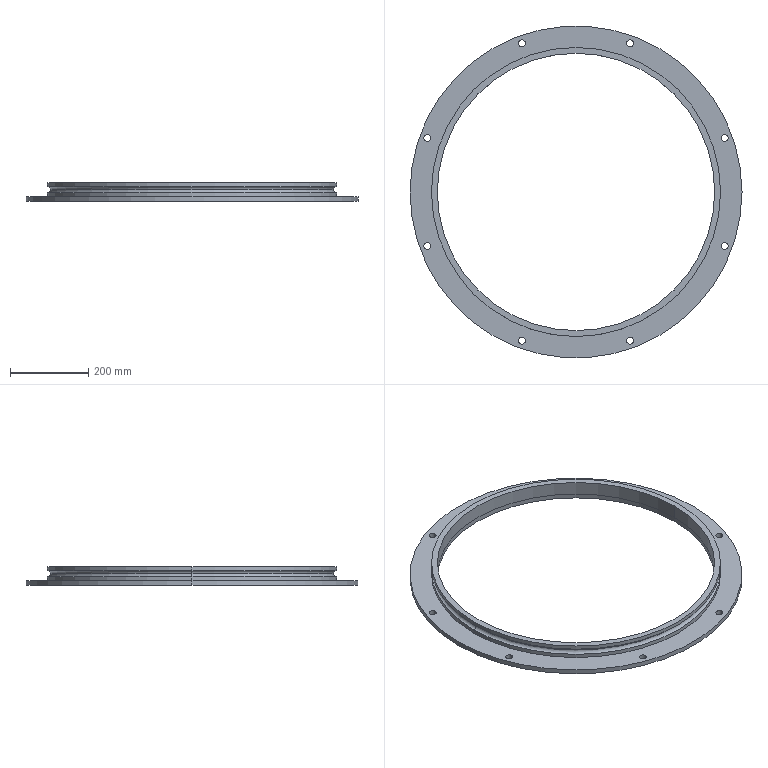Part | SolidWorks | features ICE 2, Extrusion 1, SweepCut 1 | 2 solids | 34 faces | box 850 x 850 x 48 mm | volume 3032308 mm3 | cylinder 26 | torus 4 | plane 4 | commonest cylinder face diameters 18 x16 710 x4 740 x4 850 x2
STEP:
#1=CARTESIAN_POINT('',(-370.,0.,22.));
#2=VERTEX_POINT('',#1);
#3=CARTESIAN_POINT('',(-362.,0.,30.));
#4=VERTEX_POINT('',#3);
#5=CARTESIAN_POINT('',(-370.,0.,30.));
#6=DIRECTION('',(0.,-1.,0.));
#7=DIRECTION('',(0.,0.,-1.));
#8=AXIS2_PLACEMENT_3D('',#5,#6,#7);
#9=CIRCLE('',#8,8.);
#10=EDGE_CURVE('',#2,#4,#9,.T.);
#11=ORIENTED_EDGE('',*,*,#10,.T.);
#12=CARTESIAN_POINT('',(362.,0.,30.));
#13=VERTEX_POINT('',#12);
#14=CARTESIAN_POINT('',(0.,0.,30.));
#15=DIRECTION('',(0.,0.,-1.));
#16=DIRECTION('',(-1.,0.,0.));
#17=AXIS2_PLACEMENT_3D('',#14,#15,#16);
#18=CIRCLE('',#17,362.);
#19=EDGE_CURVE('',#4,#13,#18,.T.);
#20=ORIENTED_EDGE('',*,*,#19,.T.);
#21=CARTESIAN_POINT('',(370.,0.,22.));
#22=VERTEX_POINT('',#21);
#23=CARTESIAN_POINT('',(370.,0.,30.));
#24=DIRECTION('',(0.,1.,0.));
#25=DIRECTION('',(-1.,0.,0.));
#26=AXIS2_PLACEMENT_3D('',#23,#24,#25);
#27=CIRCLE('',#26,8.);
#28=EDGE_CURVE('',#22,#13,#27,.T.);
#29=ORIENTED_EDGE('',*,*,#28,.F.);
#30=CARTESIAN_POINT('',(0.,0.,22.));
#31=DIRECTION('',(0.,0.,-1.));
#32=DIRECTION('',(1.,0.,0.));
#33=AXIS2_PLACEMENT_3D('',#30,#31,#32);
#34=CIRCLE('',#33,370.);
#35=EDGE_CURVE('',#2,#22,#34,.T.);
#36=ORIENTED_EDGE('',*,*,#35,.F.);
#37=EDGE_LOOP('',(#11,#20,#29,#36));
#38=FACE_OUTER_BOUND('',#37,.T.);
#39=CARTESIAN_POINT('',(0.,0.,30.));
#40=DIRECTION('',(0.,0.,-1.));
#41=DIRECTION('',(-1.,0.,0.));
#42=AXIS2_PLACEMENT_3D('',#39,#40,#41);
#43=TOROIDAL_SURFACE('',#42,370.,8.);
#44=ADVANCED_FACE('',(#38),#43,.F.);
#45=ORIENTED_EDGE('',*,*,#28,.T.);
#46=CARTESIAN_POINT('',(0.,0.,30.));
#47=DIRECTION('',(0.,0.,-1.));
#48=DIRECTION('',(-1.,0.,0.));
#49=AXIS2_PLACEMENT_3D('',#46,#47,#48);
#50=CIRCLE('',#49,362.);
#51=EDGE_CURVE('',#13,#4,#50,.T.);
#52=ORIENTED_EDGE('',*,*,#51,.T.);
#53=ORIENTED_EDGE('',*,*,#10,.F.);
#54=CARTESIAN_POINT('',(0.,0.,22.));
#55=DIRECTION('',(0.,0.,-1.));
#56=DIRECTION('',(1.,0.,0.));
#57=AXIS2_PLACEMENT_3D('',#54,#55,#56);
#58=CIRCLE('',#57,370.);
#59=EDGE_CURVE('',#22,#2,#58,.T.);
#60=ORIENTED_EDGE('',*,*,#59,.F.);
#61=EDGE_LOOP('',(#45,#52,#53,#60));
#62=FACE_OUTER_BOUND('',#61,.T.);
#63=CARTESIAN_POINT('',(0.,0.,30.));
#64=DIRECTION('',(0.,0.,-1.));
#65=DIRECTION('',(-1.,0.,0.));
#66=AXIS2_PLACEMENT_3D('',#63,#64,#65);
#67=TOROIDAL_SURFACE('',#66,370.,8.);
#68=ADVANCED_FACE('',(#62),#67,.F.);
#69=ORIENTED_EDGE('',*,*,#51,.F.);
#70=CARTESIAN_POINT('',(370.,0.,38.));
#71=VERTEX_POINT('',#70);
#72=CARTESIAN_POINT('',(370.,0.,30.));
#73=DIRECTION('',(0.,1.,0.));
#74=DIRECTION('',(-1.,0.,0.));
#75=AXIS2_PLACEMENT_3D('',#72,#73,#74);
#76=CIRCLE('',#75,8.);
#77=EDGE_CURVE('',#13,#71,#76,.T.);
#78=ORIENTED_EDGE('',*,*,#77,.T.);
#79=CARTESIAN_POINT('',(-370.,0.,38.));
#80=VERTEX_POINT('',#79);
#81=CARTESIAN_POINT('',(0.,0.,38.));
#82=DIRECTION('',(0.,0.,1.));
#83=DIRECTION('',(-1.,0.,0.));
#84=AXIS2_PLACEMENT_3D('',#81,#82,#83);
#85=CIRCLE('',#84,370.);
#86=EDGE_CURVE('',#80,#71,#85,.T.);
#87=ORIENTED_EDGE('',*,*,#86,.F.);
#88=CARTESIAN_POINT('',(-370.,0.,30.));
#89=DIRECTION('',(0.,-1.,0.));
#90=DIRECTION('',(0.,0.,-1.));
#91=AXIS2_PLACEMENT_3D('',#88,#89,#90);
#92=CIRCLE('',#91,8.);
#93=EDGE_CURVE('',#4,#80,#92,.T.);
#94=ORIENTED_EDGE('',*,*,#93,.F.);
#95=EDGE_LOOP('',(#69,#78,#87,#94));
#96=FACE_OUTER_BOUND('',#95,.T.);
#97=CARTESIAN_POINT('',(0.,0.,30.));
#98=DIRECTION('',(0.,0.,-1.));
#99=DIRECTION('',(-1.,0.,0.));
#100=AXIS2_PLACEMENT_3D('',#97,#98,#99);
#101=TOROIDAL_SURFACE('',#100,370.,8.);
#102=ADVANCED_FACE('',(#96),#101,.F.);
#103=CARTESIAN_POINT('',(-355.,0.,48.));
#104=VERTEX_POINT('',#103);
#105=CARTESIAN_POINT('',(355.,0.,48.));
#106=VERTEX_POINT('',#105);
#107=CARTESIAN_POINT('',(0.,0.,48.));
#108=DIRECTION('',(0.,0.,1.));
#109=DIRECTION('',(1.,0.,0.));
#110=AXIS2_PLACEMENT_3D('',#107,#108,#109);
#111=CIRCLE('',#110,355.);
#112=EDGE_CURVE('',#104,#106,#111,.T.);
#113=ORIENTED_EDGE('',*,*,#112,.T.);
#114=CARTESIAN_POINT('',(355.,0.,12.));
#115=VERTEX_POINT('',#114);
#116=CARTESIAN_POINT('',(355.,0.,48.));
#117=DIRECTION('',(0.,0.,-1.));
#118=VECTOR('',#117,1000.);
#119=LINE('',#116,#118);
#120=EDGE_CURVE('',#106,#115,#119,.T.);
#121=ORIENTED_EDGE('',*,*,#120,.T.);
#122=CARTESIAN_POINT('',(-355.,0.,12.));
#123=VERTEX_POINT('',#122);
#124=CARTESIAN_POINT('',(0.,0.,12.));
#125=DIRECTION('',(0.,0.,1.));
#126=DIRECTION('',(1.,0.,0.));
#127=AXIS2_PLACEMENT_3D('',#124,#125,#126);
#128=CIRCLE('',#127,355.);
#129=EDGE_CURVE('',#123,#115,#128,.T.);
#130=ORIENTED_EDGE('',*,*,#129,.F.);
#131=CARTESIAN_POINT('',(-355.,0.,48.));
#132=DIRECTION('',(0.,0.,-1.));
#133=VECTOR('',#132,1000.);
#134=LINE('',#131,#133);
#135=EDGE_CURVE('',#104,#123,#134,.T.);
#136=ORIENTED_EDGE('',*,*,#135,.F.);
#137=EDGE_LOOP('',(#113,#121,#130,#136));
#138=FACE_OUTER_BOUND('',#137,.T.);
#139=CARTESIAN_POINT('',(0.,0.,48.));
#140=DIRECTION('',(0.,0.,-1.));
#141=DIRECTION('',(-1.,0.,0.));
#142=AXIS2_PLACEMENT_3D('',#139,#140,#141);
#143=CYLINDRICAL_SURFACE('',#142,355.);
#144=ADVANCED_FACE('',(#138),#143,.F.);
#145=CARTESIAN_POINT('',(370.,0.,48.));
#146=VERTEX_POINT('',#145);
#147=CARTESIAN_POINT('',(-370.,0.,48.));
#148=VERTEX_POINT('',#147);
#149=CARTESIAN_POINT('',(0.,0.,48.));
#150=DIRECTION('',(0.,0.,1.));
#151=DIRECTION('',(1.,0.,0.));
#152=AXIS2_PLACEMENT_3D('',#149,#150,#151);
#153=CIRCLE('',#152,370.);
#154=EDGE_CURVE('',#146,#148,#153,.T.);
#155=ORIENTED_EDGE('',*,*,#154,.F.);
#156=CARTESIAN_POINT('',(370.,0.,48.));
#157=DIRECTION('',(0.,0.,-1.));
#158=VECTOR('',#157,1000.);
#159=LINE('',#156,#158);
#160=EDGE_CURVE('',#146,#71,#159,.T.);
#161=ORIENTED_EDGE('',*,*,#160,.T.);
#162=CARTESIAN_POINT('',(0.,0.,38.));
#163=DIRECTION('',(0.,0.,1.));
#164=DIRECTION('',(-1.,0.,0.));
#165=AXIS2_PLACEMENT_3D('',#162,#163,#164);
#166=CIRCLE('',#165,370.);
#167=EDGE_CURVE('',#71,#80,#166,.T.);
#168=ORIENTED_EDGE('',*,*,#167,.T.);
#169=CARTESIAN_POINT('',(-370.,0.,48.));
#170=DIRECTION('',(0.,0.,-1.));
#171=VECTOR('',#170,1000.);
#172=LINE('',#169,#171);
#173=EDGE_CURVE('',#148,#80,#172,.T.);
#174=ORIENTED_EDGE('',*,*,#173,.F.);
#175=EDGE_LOOP('',(#155,#161,#168,#174));
#176=FACE_OUTER_BOUND('',#175,.T.);
#177=CARTESIAN_POINT('',(0.,0.,48.));
#178=DIRECTION('',(0.,0.,-1.));
#179=DIRECTION('',(-1.,0.,0.));
#180=AXIS2_PLACEMENT_3D('',#177,#178,#179);
#181=CYLINDRICAL_SURFACE('',#180,370.);
#182=ADVANCED_FACE('',(#176),#181,.T.);
#183=ORIENTED_EDGE('',*,*,#35,.T.);
#184=CARTESIAN_POINT('',(370.,0.,12.));
#185=VERTEX_POINT('',#184);
#186=CARTESIAN_POINT('',(370.,0.,48.));
#187=DIRECTION('',(0.,0.,-1.));
#188=VECTOR('',#187,1000.);
#189=LINE('',#186,#188);
#190=EDGE_CURVE('',#22,#185,#189,.T.);
#191=ORIENTED_EDGE('',*,*,#190,.T.);
#192=CARTESIAN_POINT('',(-370.,0.,12.));
#193=VERTEX_POINT('',#192);
#194=CARTESIAN_POINT('',(0.,0.,12.));
#195=DIRECTION('',(0.,0.,1.));
#196=DIRECTION('',(1.,0.,0.));
#197=AXIS2_PLACEMENT_3D('',#194,#195,#196);
#198=CIRCLE('',#197,370.);
#199=EDGE_CURVE('',#185,#193,#198,.T.);
#200=ORIENTED_EDGE('',*,*,#199,.T.);
#201=CARTESIAN_POINT('',(-370.,0.,48.));
#202=DIRECTION('',(0.,0.,-1.));
#203=VECTOR('',#202,1000.);
#204=LINE('',#201,#203);
#205=EDGE_CURVE('',#2,#193,#204,.T.);
#206=ORIENTED_EDGE('',*,*,#205,.F.);
#207=EDGE_LOOP('',(#183,#191,#200,#206));
#208=FACE_OUTER_BOUND('',#207,.T.);
#209=CARTESIAN_POINT('',(0.,0.,48.));
#210=DIRECTION('',(0.,0.,-1.));
#211=DIRECTION('',(-1.,0.,0.));
#212=AXIS2_PLACEMENT_3D('',#209,#210,#211);
#213=CYLINDRICAL_SURFACE('',#212,370.);
#214=ADVANCED_FACE('',(#208),#213,.T.);
#215=ORIENTED_EDGE('',*,*,#190,.F.);
#216=ORIENTED_EDGE('',*,*,#59,.T.);
#217=ORIENTED_EDGE('',*,*,#205,.T.);
#218=CARTESIAN_POINT('',(0.,0.,12.));
#219=DIRECTION('',(0.,0.,1.));
#220=DIRECTION('',(1.,0.,0.));
#221=AXIS2_PLACEMENT_3D('',#218,#219,#220);
#222=CIRCLE('',#221,370.);
#223=EDGE_CURVE('',#193,#185,#222,.T.);
#224=ORIENTED_EDGE('',*,*,#223,.T.);
#225=EDGE_LOOP('',(#215,#216,#217,#224));
#226=FACE_OUTER_BOUND('',#225,.T.);
#227=CARTESIAN_POINT('',(0.,0.,48.));
#228=DIRECTION('',(0.,0.,-1.));
#229=DIRECTION('',(-1.,0.,0.));
#230=AXIS2_PLACEMENT_3D('',#227,#228,#229);
#231=CYLINDRICAL_SURFACE('',#230,370.);
#232=ADVANCED_FACE('',(#226),#231,.T.);
#233=CARTESIAN_POINT('',(0.,0.,48.));
#234=DIRECTION('',(0.,0.,1.));
#235=DIRECTION('',(1.,0.,0.));
#236=AXIS2_PLACEMENT_3D('',#233,#234,#235);
#237=CIRCLE('',#236,370.);
#238=EDGE_CURVE('',#148,#146,#237,.T.);
#239=ORIENTED_EDGE('',*,*,#238,.T.);
#240=ORIENTED_EDGE('',*,*,#154,.T.);
#241=EDGE_LOOP('',(#239,#240));
#242=FACE_OUTER_BOUND('',#241,.T.);
#243=ORIENTED_EDGE('',*,*,#112,.F.);
#244=CARTESIAN_POINT('',(0.,0.,48.));
#245=DIRECTION('',(0.,0.,1.));
#246=DIRECTION('',(1.,0.,0.));
#247=AXIS2_PLACEMENT_3D('',#244,#245,#246);
#248=CIRCLE('',#247,355.);
#249=EDGE_CURVE('',#106,#104,#248,.T.);
#250=ORIENTED_EDGE('',*,*,#249,.F.);
#251=EDGE_LOOP('',(#243,#250));
#252=FACE_BOUND('',#251,.T.);
#253=CARTESIAN_POINT('',(0.,0.,48.));
#254=DIRECTION('',(0.,0.,1.));
#255=DIRECTION('',(1.,0.,0.));
#256=AXIS2_PLACEMENT_3D('',#253,#254,#255);
#257=PLANE('',#256);
#258=ADVANCED_FACE('',(#242,#252),#257,.T.);
#259=ORIENTED_EDGE('',*,*,#223,.F.);
#260=ORIENTED_EDGE('',*,*,#199,.F.);
#261=EDGE_LOOP('',(#259,#260));
#262=FACE_OUTER_BOUND('',#261,.T.);
#263=ORIENTED_EDGE('',*,*,#129,.T.);
#264=CARTESIAN_POINT('',(0.,0.,12.));
#265=DIRECTION('',(0.,0.,1.));
#266=DIRECTION('',(1.,0.,0.));
#267=AXIS2_PLACEMENT_3D('',#264,#265,#266);
#268=CIRCLE('',#267,355.);
#269=EDGE_CURVE('',#115,#123,#268,.T.);
#270=ORIENTED_EDGE('',*,*,#269,.T.);
#271=EDGE_LOOP('',(#263,#270));
#272=FACE_BOUND('',#271,.T.);
#273=CARTESIAN_POINT('',(0.,0.,12.));
#274=DIRECTION('',(0.,0.,1.));
#275=DIRECTION('',(1.,0.,0.));
#276=AXIS2_PLACEMENT_3D('',#273,#274,#275);
#277=PLANE('',#276);
#278=ADVANCED_FACE('',(#262,#272),#277,.F.);
#279=ORIENTED_EDGE('',*,*,#160,.F.);
#280=ORIENTED_EDGE('',*,*,#238,.F.);
#281=ORIENTED_EDGE('',*,*,#173,.T.);
#282=ORIENTED_EDGE('',*,*,#86,.T.);
#283=EDGE_LOOP('',(#279,#280,#281,#282));
#284=FACE_OUTER_BOUND('',#283,.T.);
#285=CARTESIAN_POINT('',(0.,0.,48.));
#286=DIRECTION('',(0.,0.,-1.));
#287=DIRECTION('',(-1.,0.,0.));
#288=AXIS2_PLACEMENT_3D('',#285,#286,#287);
#289=CYLINDRICAL_SURFACE('',#288,370.);
#290=ADVANCED_FACE('',(#284),#289,.T.);
#291=ORIENTED_EDGE('',*,*,#120,.F.);
#292=ORIENTED_EDGE('',*,*,#249,.T.);
#293=ORIENTED_EDGE('',*,*,#135,.T.);
#294=ORIENTED_EDGE('',*,*,#269,.F.);
#295=EDGE_LOOP('',(#291,#292,#293,#294));
#296=FACE_OUTER_BOUND('',#295,.T.);
#297=CARTESIAN_POINT('',(0.,0.,48.));
#298=DIRECTION('',(0.,0.,-1.));
#299=DIRECTION('',(-1.,0.,0.));
#300=AXIS2_PLACEMENT_3D('',#297,#298,#299);
#301=CYLINDRICAL_SURFACE('',#300,355.);
#302=ADVANCED_FACE('',(#296),#301,.F.);
#303=ORIENTED_EDGE('',*,*,#19,.F.);
#304=ORIENTED_EDGE('',*,*,#93,.T.);
#305=ORIENTED_EDGE('',*,*,#167,.F.);
#306=ORIENTED_EDGE('',*,*,#77,.F.);
#307=EDGE_LOOP('',(#303,#304,#305,#306));
#308=FACE_OUTER_BOUND('',#307,.T.);
#309=CARTESIAN_POINT('',(0.,0.,30.));
#310=DIRECTION('',(0.,0.,-1.));
#311=DIRECTION('',(-1.,0.,0.));
#312=AXIS2_PLACEMENT_3D('',#309,#310,#311);
#313=TOROIDAL_SURFACE('',#312,370.,8.);
#314=ADVANCED_FACE('',(#308),#313,.F.);
#315=CLOSED_SHELL('',(#44,#68,#102,#144,#182,#214,#232,#258,#278,#290,#302,#314));
#316=MANIFOLD_SOLID_BREP('',#315);
#317=CARTESIAN_POINT('',(129.5,380.582,0.));
#318=VERTEX_POINT('',#317);
#319=CARTESIAN_POINT('',(147.5,380.582,0.));
#320=VERTEX_POINT('',#319);
#321=CARTESIAN_POINT('',(138.5,380.582,0.));
#322=DIRECTION('',(0.,0.,1.));
#323=DIRECTION('',(1.,0.,0.));
#324=AXIS2_PLACEMENT_3D('',#321,#322,#323);
#325=CIRCLE('',#324,9.);
#326=EDGE_CURVE('',#318,#320,#325,.T.);
#327=ORIENTED_EDGE('',*,*,#326,.F.);
#328=CARTESIAN_POINT('',(129.5,380.582,12.));
#329=VERTEX_POINT('',#328);
#330=CARTESIAN_POINT('',(129.5,380.582,-8.));
#331=DIRECTION('',(0.,0.,1.));
#332=VECTOR('',#331,1000.);
#333=LINE('',#330,#332);
#334=EDGE_CURVE('',#318,#329,#333,.T.);
#335=ORIENTED_EDGE('',*,*,#334,.T.);
#336=CARTESIAN_POINT('',(147.5,380.582,12.));
#337=VERTEX_POINT('',#336);
#338=CARTESIAN_POINT('',(138.5,380.582,12.));
#339=DIRECTION('',(0.,0.,1.));
#340=DIRECTION('',(1.,0.,0.));
#341=AXIS2_PLACEMENT_3D('',#338,#339,#340);
#342=CIRCLE('',#341,9.);
#343=EDGE_CURVE('',#329,#337,#342,.T.);
#344=ORIENTED_EDGE('',*,*,#343,.T.);
#345=CARTESIAN_POINT('',(147.5,380.582,-8.));
#346=DIRECTION('',(0.,0.,1.));
#347=VECTOR('',#346,1000.);
#348=LINE('',#345,#347);
#349=EDGE_CURVE('',#320,#337,#348,.T.);
#350=ORIENTED_EDGE('',*,*,#349,.F.);
#351=EDGE_LOOP('',(#327,#335,#344,#350));
#352=FACE_OUTER_BOUND('',#351,.T.);
#353=CARTESIAN_POINT('',(138.5,380.582,-8.));
#354=DIRECTION('',(0.,0.,1.));
#355=DIRECTION('',(1.,0.,0.));
#356=AXIS2_PLACEMENT_3D('',#353,#354,#355);
#357=CYLINDRICAL_SURFACE('',#356,9.);
#358=ADVANCED_FACE('',(#352),#357,.F.);
#359=CARTESIAN_POINT('',(129.5,-380.582,0.));
#360=VERTEX_POINT('',#359);
#361=CARTESIAN_POINT('',(147.5,-380.582,0.));
#362=VERTEX_POINT('',#361);
#363=CARTESIAN_POINT('',(138.5,-380.582,0.));
#364=DIRECTION('',(0.,0.,1.));
#365=DIRECTION('',(1.,0.,0.));
#366=AXIS2_PLACEMENT_3D('',#363,#364,#365);
#367=CIRCLE('',#366,9.);
#368=EDGE_CURVE('',#360,#362,#367,.T.);
#369=ORIENTED_EDGE('',*,*,#368,.F.);
#370=CARTESIAN_POINT('',(129.5,-380.582,12.));
#371=VERTEX_POINT('',#370);
#372=CARTESIAN_POINT('',(129.5,-380.582,-8.));
#373=DIRECTION('',(0.,0.,1.));
#374=VECTOR('',#373,1000.);
#375=LINE('',#372,#374);
#376=EDGE_CURVE('',#360,#371,#375,.T.);
#377=ORIENTED_EDGE('',*,*,#376,.T.);
#378=CARTESIAN_POINT('',(147.5,-380.582,12.));
#379=VERTEX_POINT('',#378);
#380=CARTESIAN_POINT('',(138.5,-380.582,12.));
#381=DIRECTION('',(0.,0.,1.));
#382=DIRECTION('',(-1.,0.,0.));
#383=AXIS2_PLACEMENT_3D('',#380,#381,#382);
#384=CIRCLE('',#383,9.);
#385=EDGE_CURVE('',#371,#379,#384,.T.);
#386=ORIENTED_EDGE('',*,*,#385,.T.);
#387=CARTESIAN_POINT('',(147.5,-380.582,-8.));
#388=DIRECTION('',(0.,0.,1.));
#389=VECTOR('',#388,1000.);
#390=LINE('',#387,#389);
#391=EDGE_CURVE('',#362,#379,#390,.T.);
#392=ORIENTED_EDGE('',*,*,#391,.F.);
#393=EDGE_LOOP('',(#369,#377,#386,#392));
#394=FACE_OUTER_BOUND('',#393,.T.);
#395=CARTESIAN_POINT('',(138.5,-380.582,-8.));
#396=DIRECTION('',(0.,0.,1.));
#397=DIRECTION('',(1.,0.,0.));
#398=AXIS2_PLACEMENT_3D('',#395,#396,#397);
#399=CYLINDRICAL_SURFACE('',#398,9.);
#400=ADVANCED_FACE('',(#394),#399,.F.);
#401=CARTESIAN_POINT('',(-147.5,-380.582,0.));
#402=VERTEX_POINT('',#401);
#403=CARTESIAN_POINT('',(-129.5,-380.582,0.));
#404=VERTEX_POINT('',#403);
#405=CARTESIAN_POINT('',(-138.5,-380.582,0.));
#406=DIRECTION('',(0.,0.,1.));
#407=DIRECTION('',(1.,0.,0.));
#408=AXIS2_PLACEMENT_3D('',#405,#406,#407);
#409=CIRCLE('',#408,9.);
#410=EDGE_CURVE('',#402,#404,#409,.T.);
#411=ORIENTED_EDGE('',*,*,#410,.F.);
#412=CARTESIAN_POINT('',(-147.5,-380.582,12.));
#413=VERTEX_POINT('',#412);
#414=CARTESIAN_POINT('',(-147.5,-380.582,-8.));
#415=DIRECTION('',(0.,0.,1.));
#416=VECTOR('',#415,1000.);
#417=LINE('',#414,#416);
#418=EDGE_CURVE('',#402,#413,#417,.T.);
#419=ORIENTED_EDGE('',*,*,#418,.T.);
#420=CARTESIAN_POINT('',(-129.5,-380.582,12.));
#421=VERTEX_POINT('',#420);
#422=CARTESIAN_POINT('',(-138.5,-380.582,12.));
#423=DIRECTION('',(0.,0.,1.));
#424=DIRECTION('',(-1.,0.,0.));
#425=AXIS2_PLACEMENT_3D('',#422,#423,#424);
#426=CIRCLE('',#425,9.);
#427=EDGE_CURVE('',#413,#421,#426,.T.);
#428=ORIENTED_EDGE('',*,*,#427,.T.);
#429=CARTESIAN_POINT('',(-129.5,-380.582,-8.));
#430=DIRECTION('',(0.,0.,1.));
#431=VECTOR('',#430,1000.);
#432=LINE('',#429,#431);
#433=EDGE_CURVE('',#404,#421,#432,.T.);
#434=ORIENTED_EDGE('',*,*,#433,.F.);
#435=EDGE_LOOP('',(#411,#419,#428,#434));
#436=FACE_OUTER_BOUND('',#435,.T.);
#437=CARTESIAN_POINT('',(-138.5,-380.582,-8.));
#438=DIRECTION('',(0.,0.,1.));
#439=DIRECTION('',(1.,0.,0.));
#440=AXIS2_PLACEMENT_3D('',#437,#438,#439);
#441=CYLINDRICAL_SURFACE('',#440,9.);
#442=ADVANCED_FACE('',(#436),#441,.F.);
#443=CARTESIAN_POINT('',(-389.582,138.5,0.));
#444=VERTEX_POINT('',#443);
#445=CARTESIAN_POINT('',(-371.582,138.5,0.));
#446=VERTEX_POINT('',#445);
#447=CARTESIAN_POINT('',(-380.582,138.5,0.));
#448=DIRECTION('',(0.,0.,1.));
#449=DIRECTION('',(1.,0.,0.));
#450=AXIS2_PLACEMENT_3D('',#447,#448,#449);
#451=CIRCLE('',#450,9.);
#452=EDGE_CURVE('',#444,#446,#451,.T.);
#453=ORIENTED_EDGE('',*,*,#452,.F.);
#454=CARTESIAN_POINT('',(-389.582,138.5,12.));
#455=VERTEX_POINT('',#454);
#456=CARTESIAN_POINT('',(-389.582,138.5,-8.));
#457=DIRECTION('',(0.,0.,1.));
#458=VECTOR('',#457,1000.);
#459=LINE('',#456,#458);
#460=EDGE_CURVE('',#444,#455,#459,.T.);
#461=ORIENTED_EDGE('',*,*,#460,.T.);
#462=CARTESIAN_POINT('',(-371.582,138.5,12.));
#463=VERTEX_POINT('',#462);
#464=CARTESIAN_POINT('',(-380.582,138.5,12.));
#465=DIRECTION('',(0.,0.,1.));
#466=DIRECTION('',(1.,0.,0.));
#467=AXIS2_PLACEMENT_3D('',#464,#465,#466);
#468=CIRCLE('',#467,9.);
#469=EDGE_CURVE('',#455,#463,#468,.T.);
#470=ORIENTED_EDGE('',*,*,#469,.T.);
#471=CARTESIAN_POINT('',(-371.582,138.5,-8.));
#472=DIRECTION('',(0.,0.,1.));
#473=VECTOR('',#472,1000.);
#474=LINE('',#471,#473);
#475=EDGE_CURVE('',#446,#463,#474,.T.);
#476=ORIENTED_EDGE('',*,*,#475,.F.);
#477=EDGE_LOOP('',(#453,#461,#470,#476));
#478=FACE_OUTER_BOUND('',#477,.T.);
#479=CARTESIAN_POINT('',(-380.582,138.5,-8.));
#480=DIRECTION('',(0.,0.,1.));
#481=DIRECTION('',(1.,0.,0.));
#482=AXIS2_PLACEMENT_3D('',#479,#480,#481);
#483=CYLINDRICAL_SURFACE('',#482,9.);
#484=ADVANCED_FACE('',(#478),#483,.F.);
#485=CARTESIAN_POINT('',(-389.582,-138.5,0.));
#486=VERTEX_POINT('',#485);
#487=CARTESIAN_POINT('',(-371.582,-138.5,0.));
#488=VERTEX_POINT('',#487);
#489=CARTESIAN_POINT('',(-380.582,-138.5,0.));
#490=DIRECTION('',(0.,0.,1.));
#491=DIRECTION('',(1.,0.,0.));
#492=AXIS2_PLACEMENT_3D('',#489,#490,#491);
#493=CIRCLE('',#492,9.);
#494=EDGE_CURVE('',#486,#488,#493,.T.);
#495=ORIENTED_EDGE('',*,*,#494,.F.);
#496=CARTESIAN_POINT('',(-389.582,-138.5,12.));
#497=VERTEX_POINT('',#496);
#498=CARTESIAN_POINT('',(-389.582,-138.5,-8.));
#499=DIRECTION('',(0.,0.,1.));
#500=VECTOR('',#499,1000.);
#501=LINE('',#498,#500);
#502=EDGE_CURVE('',#486,#497,#501,.T.);
#503=ORIENTED_EDGE('',*,*,#502,.T.);
#504=CARTESIAN_POINT('',(-371.582,-138.5,12.));
#505=VERTEX_POINT('',#504);
#506=CARTESIAN_POINT('',(-380.582,-138.5,12.));
#507=DIRECTION('',(0.,0.,1.));
#508=DIRECTION('',(1.,0.,0.));
#509=AXIS2_PLACEMENT_3D('',#506,#507,#508);
#510=CIRCLE('',#509,9.);
#511=EDGE_CURVE('',#497,#505,#510,.T.);
#512=ORIENTED_EDGE('',*,*,#511,.T.);
#513=CARTESIAN_POINT('',(-371.582,-138.5,-8.));
#514=DIRECTION('',(0.,0.,1.));
#515=VECTOR('',#514,1000.);
#516=LINE('',#513,#515);
#517=EDGE_CURVE('',#488,#505,#516,.T.);
#518=ORIENTED_EDGE('',*,*,#517,.F.);
#519=EDGE_LOOP('',(#495,#503,#512,#518));
#520=FACE_OUTER_BOUND('',#519,.T.);
#521=CARTESIAN_POINT('',(-380.582,-138.5,-8.));
#522=DIRECTION('',(0.,0.,1.));
#523=DIRECTION('',(1.,0.,0.));
#524=AXIS2_PLACEMENT_3D('',#521,#522,#523);
#525=CYLINDRICAL_SURFACE('',#524,9.);
#526=ADVANCED_FACE('',(#520),#525,.F.);
#527=CARTESIAN_POINT('',(371.582,-138.5,0.));
#528=VERTEX_POINT('',#527);
#529=CARTESIAN_POINT('',(389.582,-138.5,0.));
#530=VERTEX_POINT('',#529);
#531=CARTESIAN_POINT('',(380.582,-138.5,0.));
#532=DIRECTION('',(0.,0.,1.));
#533=DIRECTION('',(1.,0.,0.));
#534=AXIS2_PLACEMENT_3D('',#531,#532,#533);
#535=CIRCLE('',#534,9.);
#536=EDGE_CURVE('',#528,#530,#535,.T.);
#537=ORIENTED_EDGE('',*,*,#536,.F.);
#538=CARTESIAN_POINT('',(371.582,-138.5,12.));
#539=VERTEX_POINT('',#538);
#540=CARTESIAN_POINT('',(371.582,-138.5,-8.));
#541=DIRECTION('',(0.,0.,1.));
#542=VECTOR('',#541,1000.);
#543=LINE('',#540,#542);
#544=EDGE_CURVE('',#528,#539,#543,.T.);
#545=ORIENTED_EDGE('',*,*,#544,.T.);
#546=CARTESIAN_POINT('',(389.582,-138.5,12.));
#547=VERTEX_POINT('',#546);
#548=CARTESIAN_POINT('',(380.582,-138.5,12.));
#549=DIRECTION('',(0.,0.,1.));
#550=DIRECTION('',(-1.,0.,0.));
#551=AXIS2_PLACEMENT_3D('',#548,#549,#550);
#552=CIRCLE('',#551,9.);
#553=EDGE_CURVE('',#539,#547,#552,.T.);
#554=ORIENTED_EDGE('',*,*,#553,.T.);
#555=CARTESIAN_POINT('',(389.582,-138.5,-8.));
#556=DIRECTION('',(0.,0.,1.));
#557=VECTOR('',#556,1000.);
#558=LINE('',#555,#557);
#559=EDGE_CURVE('',#530,#547,#558,.T.);
#560=ORIENTED_EDGE('',*,*,#559,.F.);
#561=EDGE_LOOP('',(#537,#545,#554,#560));
#562=FACE_OUTER_BOUND('',#561,.T.);
#563=CARTESIAN_POINT('',(380.582,-138.5,-8.));
#564=DIRECTION('',(0.,0.,1.));
#565=DIRECTION('',(1.,0.,0.));
#566=AXIS2_PLACEMENT_3D('',#563,#564,#565);
#567=CYLINDRICAL_SURFACE('',#566,9.);
#568=ADVANCED_FACE('',(#562),#567,.F.);
#569=CARTESIAN_POINT('',(371.582,138.5,0.));
#570=VERTEX_POINT('',#569);
#571=CARTESIAN_POINT('',(389.582,138.5,0.));
#572=VERTEX_POINT('',#571);
#573=CARTESIAN_POINT('',(380.582,138.5,0.));
#574=DIRECTION('',(0.,0.,1.));
#575=DIRECTION('',(1.,0.,0.));
#576=AXIS2_PLACEMENT_3D('',#573,#574,#575);
#577=CIRCLE('',#576,9.);
#578=EDGE_CURVE('',#570,#572,#577,.T.);
#579=ORIENTED_EDGE('',*,*,#578,.F.);
#580=CARTESIAN_POINT('',(371.582,138.5,12.));
#581=VERTEX_POINT('',#580);
#582=CARTESIAN_POINT('',(371.582,138.5,-8.));
#583=DIRECTION('',(0.,0.,1.));
#584=VECTOR('',#583,1000.);
#585=LINE('',#582,#584);
#586=EDGE_CURVE('',#570,#581,#585,.T.);
#587=ORIENTED_EDGE('',*,*,#586,.T.);
#588=CARTESIAN_POINT('',(389.582,138.5,12.));
#589=VERTEX_POINT('',#588);
#590=CARTESIAN_POINT('',(380.582,138.5,12.));
#591=DIRECTION('',(0.,0.,1.));
#592=DIRECTION('',(-1.,0.,0.));
#593=AXIS2_PLACEMENT_3D('',#590,#591,#592);
#594=CIRCLE('',#593,9.);
#595=EDGE_CURVE('',#581,#589,#594,.T.);
#596=ORIENTED_EDGE('',*,*,#595,.T.);
#597=CARTESIAN_POINT('',(389.582,138.5,-8.));
#598=DIRECTION('',(0.,0.,1.));
#599=VECTOR('',#598,1000.);
#600=LINE('',#597,#599);
#601=EDGE_CURVE('',#572,#589,#600,.T.);
#602=ORIENTED_EDGE('',*,*,#601,.F.);
#603=EDGE_LOOP('',(#579,#587,#596,#602));
#604=FACE_OUTER_BOUND('',#603,.T.);
#605=CARTESIAN_POINT('',(380.582,138.5,-8.));
#606=DIRECTION('',(0.,0.,1.));
#607=DIRECTION('',(1.,0.,0.));
#608=AXIS2_PLACEMENT_3D('',#605,#606,#607);
#609=CYLINDRICAL_SURFACE('',#608,9.);
#610=ADVANCED_FACE('',(#604),#609,.F.);
#611=CARTESIAN_POINT('',(-147.5,380.582,0.));
#612=VERTEX_POINT('',#611);
#613=CARTESIAN_POINT('',(-129.5,380.582,0.));
#614=VERTEX_POINT('',#613);
#615=CARTESIAN_POINT('',(-138.5,380.582,0.));
#616=DIRECTION('',(0.,0.,1.));
#617=DIRECTION('',(1.,0.,0.));
#618=AXIS2_PLACEMENT_3D('',#615,#616,#617);
#619=CIRCLE('',#618,9.);
#620=EDGE_CURVE('',#612,#614,#619,.T.);
#621=ORIENTED_EDGE('',*,*,#620,.F.);
#622=CARTESIAN_POINT('',(-147.5,380.582,12.));
#623=VERTEX_POINT('',#622);
#624=CARTESIAN_POINT('',(-147.5,380.582,-8.));
#625=DIRECTION('',(0.,0.,1.));
#626=VECTOR('',#625,1000.);
#627=LINE('',#624,#626);
#628=EDGE_CURVE('',#612,#623,#627,.T.);
#629=ORIENTED_EDGE('',*,*,#628,.T.);
#630=CARTESIAN_POINT('',(-129.5,380.582,12.));
#631=VERTEX_POINT('',#630);
#632=CARTESIAN_POINT('',(-138.5,380.582,12.));
#633=DIRECTION('',(0.,0.,1.));
#634=DIRECTION('',(1.,0.,0.));
#635=AXIS2_PLACEMENT_3D('',#632,#633,#634);
#636=CIRCLE('',#635,9.);
#637=EDGE_CURVE('',#623,#631,#636,.T.);
#638=ORIENTED_EDGE('',*,*,#637,.T.);
#639=CARTESIAN_POINT('',(-129.5,380.582,-8.));
#640=DIRECTION('',(0.,0.,1.));
#641=VECTOR('',#640,1000.);
#642=LINE('',#639,#641);
#643=EDGE_CURVE('',#614,#631,#642,.T.);
#644=ORIENTED_EDGE('',*,*,#643,.F.);
#645=EDGE_LOOP('',(#621,#629,#638,#644));
#646=FACE_OUTER_BOUND('',#645,.T.);
#647=CARTESIAN_POINT('',(-138.5,380.582,-8.));
#648=DIRECTION('',(0.,0.,1.));
#649=DIRECTION('',(1.,0.,0.));
#650=AXIS2_PLACEMENT_3D('',#647,#648,#649);
#651=CYLINDRICAL_SURFACE('',#650,9.);
#652=ADVANCED_FACE('',(#646),#651,.F.);
#653=CARTESIAN_POINT('',(-355.,0.,12.));
#654=VERTEX_POINT('',#653);
#655=CARTESIAN_POINT('',(355.,0.,12.));
#656=VERTEX_POINT('',#655);
#657=CARTESIAN_POINT('',(0.,0.,12.));
#658=DIRECTION('',(0.,0.,1.));
#659=DIRECTION('',(1.,0.,0.));
#660=AXIS2_PLACEMENT_3D('',#657,#658,#659);
#661=CIRCLE('',#660,355.);
#662=EDGE_CURVE('',#654,#656,#661,.T.);
#663=ORIENTED_EDGE('',*,*,#662,.T.);
#664=CARTESIAN_POINT('',(355.,0.,0.));
#665=VERTEX_POINT('',#664);
#666=CARTESIAN_POINT('',(355.,0.,12.));
#667=DIRECTION('',(0.,0.,-1.));
#668=VECTOR('',#667,1000.);
#669=LINE('',#666,#668);
#670=EDGE_CURVE('',#656,#665,#669,.T.);
#671=ORIENTED_EDGE('',*,*,#670,.T.);
#672=CARTESIAN_POINT('',(-355.,0.,0.));
#673=VERTEX_POINT('',#672);
#674=CARTESIAN_POINT('',(0.,0.,0.));
#675=DIRECTION('',(0.,0.,1.));
#676=DIRECTION('',(1.,0.,0.));
#677=AXIS2_PLACEMENT_3D('',#674,#675,#676);
#678=CIRCLE('',#677,355.);
#679=EDGE_CURVE('',#673,#665,#678,.T.);
#680=ORIENTED_EDGE('',*,*,#679,.F.);
#681=CARTESIAN_POINT('',(-355.,0.,12.));
#682=DIRECTION('',(0.,0.,-1.));
#683=VECTOR('',#682,1000.);
#684=LINE('',#681,#683);
#685=EDGE_CURVE('',#654,#673,#684,.T.);
#686=ORIENTED_EDGE('',*,*,#685,.F.);
#687=EDGE_LOOP('',(#663,#671,#680,#686));
#688=FACE_OUTER_BOUND('',#687,.T.);
#689=CARTESIAN_POINT('',(0.,0.,12.));
#690=DIRECTION('',(0.,0.,-1.));
#691=DIRECTION('',(-1.,0.,0.));
#692=AXIS2_PLACEMENT_3D('',#689,#690,#691);
#693=CYLINDRICAL_SURFACE('',#692,355.);
#694=ADVANCED_FACE('',(#688),#693,.F.);
#695=CARTESIAN_POINT('',(425.,0.,12.));
#696=VERTEX_POINT('',#695);
#697=CARTESIAN_POINT('',(-425.,0.,12.));
#698=VERTEX_POINT('',#697);
#699=CARTESIAN_POINT('',(0.,0.,12.));
#700=DIRECTION('',(0.,0.,1.));
#701=DIRECTION('',(1.,0.,0.));
#702=AXIS2_PLACEMENT_3D('',#699,#700,#701);
#703=CIRCLE('',#702,425.);
#704=EDGE_CURVE('',#696,#698,#703,.T.);
#705=ORIENTED_EDGE('',*,*,#704,.F.);
#706=CARTESIAN_POINT('',(425.,0.,0.));
#707=VERTEX_POINT('',#706);
#708=CARTESIAN_POINT('',(425.,0.,12.));
#709=DIRECTION('',(0.,0.,-1.));
#710=VECTOR('',#709,1000.);
#711=LINE('',#708,#710);
#712=EDGE_CURVE('',#696,#707,#711,.T.);
#713=ORIENTED_EDGE('',*,*,#712,.T.);
#714=CARTESIAN_POINT('',(-425.,0.,0.));
#715=VERTEX_POINT('',#714);
#716=CARTESIAN_POINT('',(0.,0.,0.));
#717=DIRECTION('',(0.,0.,1.));
#718=DIRECTION('',(1.,0.,0.));
#719=AXIS2_PLACEMENT_3D('',#716,#717,#718);
#720=CIRCLE('',#719,425.);
#721=EDGE_CURVE('',#707,#715,#720,.T.);
#722=ORIENTED_EDGE('',*,*,#721,.T.);
#723=CARTESIAN_POINT('',(-425.,0.,12.));
#724=DIRECTION('',(0.,0.,-1.));
#725=VECTOR('',#724,1000.);
#726=LINE('',#723,#725);
#727=EDGE_CURVE('',#698,#715,#726,.T.);
#728=ORIENTED_EDGE('',*,*,#727,.F.);
#729=EDGE_LOOP('',(#705,#713,#722,#728));
#730=FACE_OUTER_BOUND('',#729,.T.);
#731=CARTESIAN_POINT('',(0.,0.,12.));
#732=DIRECTION('',(0.,0.,-1.));
#733=DIRECTION('',(-1.,0.,0.));
#734=AXIS2_PLACEMENT_3D('',#731,#732,#733);
#735=CYLINDRICAL_SURFACE('',#734,425.);
#736=ADVANCED_FACE('',(#730),#735,.T.);
#737=CARTESIAN_POINT('',(138.5,380.582,12.));
#738=DIRECTION('',(0.,0.,1.));
#739=DIRECTION('',(1.,0.,0.));
#740=AXIS2_PLACEMENT_3D('',#737,#738,#739);
#741=CIRCLE('',#740,9.);
#742=EDGE_CURVE('',#337,#329,#741,.T.);
#743=ORIENTED_EDGE('',*,*,#742,.F.);
#744=ORIENTED_EDGE('',*,*,#343,.F.);
#745=EDGE_LOOP('',(#743,#744));
#746=FACE_BOUND('',#745,.T.);
#747=CARTESIAN_POINT('',(138.5,-380.582,12.));
#748=DIRECTION('',(0.,0.,1.));
#749=DIRECTION('',(-1.,0.,0.));
#750=AXIS2_PLACEMENT_3D('',#747,#748,#749);
#751=CIRCLE('',#750,9.);
#752=EDGE_CURVE('',#379,#371,#751,.T.);
#753=ORIENTED_EDGE('',*,*,#752,.F.);
#754=ORIENTED_EDGE('',*,*,#385,.F.);
#755=EDGE_LOOP('',(#753,#754));
#756=FACE_BOUND('',#755,.T.);
#757=CARTESIAN_POINT('',(-138.5,-380.582,12.));
#758=DIRECTION('',(0.,0.,1.));
#759=DIRECTION('',(-1.,0.,0.));
#760=AXIS2_PLACEMENT_3D('',#757,#758,#759);
#761=CIRCLE('',#760,9.);
#762=EDGE_CURVE('',#421,#413,#761,.T.);
#763=ORIENTED_EDGE('',*,*,#762,.F.);
#764=ORIENTED_EDGE('',*,*,#427,.F.);
#765=EDGE_LOOP('',(#763,#764));
#766=FACE_BOUND('',#765,.T.);
#767=CARTESIAN_POINT('',(-380.582,138.5,12.));
#768=DIRECTION('',(0.,0.,1.));
#769=DIRECTION('',(1.,0.,0.));
#770=AXIS2_PLACEMENT_3D('',#767,#768,#769);
#771=CIRCLE('',#770,9.);
#772=EDGE_CURVE('',#463,#455,#771,.T.);
#773=ORIENTED_EDGE('',*,*,#772,.F.);
#774=ORIENTED_EDGE('',*,*,#469,.F.);
#775=EDGE_LOOP('',(#773,#774));
#776=FACE_BOUND('',#775,.T.);
#777=CARTESIAN_POINT('',(-380.582,-138.5,12.));
#778=DIRECTION('',(0.,0.,1.));
#779=DIRECTION('',(1.,0.,0.));
#780=AXIS2_PLACEMENT_3D('',#777,#778,#779);
#781=CIRCLE('',#780,9.);
#782=EDGE_CURVE('',#505,#497,#781,.T.);
#783=ORIENTED_EDGE('',*,*,#782,.F.);
#784=ORIENTED_EDGE('',*,*,#511,.F.);
#785=EDGE_LOOP('',(#783,#784));
#786=FACE_BOUND('',#785,.T.);
#787=CARTESIAN_POINT('',(380.582,-138.5,12.));
#788=DIRECTION('',(0.,0.,1.));
#789=DIRECTION('',(-1.,0.,0.));
#790=AXIS2_PLACEMENT_3D('',#787,#788,#789);
#791=CIRCLE('',#790,9.);
#792=EDGE_CURVE('',#547,#539,#791,.T.);
#793=ORIENTED_EDGE('',*,*,#792,.F.);
#794=ORIENTED_EDGE('',*,*,#553,.F.);
#795=EDGE_LOOP('',(#793,#794));
#796=FACE_BOUND('',#795,.T.);
#797=CARTESIAN_POINT('',(380.582,138.5,12.));
#798=DIRECTION('',(0.,0.,1.));
#799=DIRECTION('',(-1.,0.,0.));
#800=AXIS2_PLACEMENT_3D('',#797,#798,#799);
#801=CIRCLE('',#800,9.);
#802=EDGE_CURVE('',#589,#581,#801,.T.);
#803=ORIENTED_EDGE('',*,*,#802,.F.);
#804=ORIENTED_EDGE('',*,*,#595,.F.);
#805=EDGE_LOOP('',(#803,#804));
#806=FACE_BOUND('',#805,.T.);
#807=CARTESIAN_POINT('',(-138.5,380.582,12.));
#808=DIRECTION('',(0.,0.,1.));
#809=DIRECTION('',(1.,0.,0.));
#810=AXIS2_PLACEMENT_3D('',#807,#808,#809);
#811=CIRCLE('',#810,9.);
#812=EDGE_CURVE('',#631,#623,#811,.T.);
#813=ORIENTED_EDGE('',*,*,#812,.F.);
#814=ORIENTED_EDGE('',*,*,#637,.F.);
#815=EDGE_LOOP('',(#813,#814));
#816=FACE_BOUND('',#815,.T.);
#817=CARTESIAN_POINT('',(0.,0.,12.));
#818=DIRECTION('',(0.,0.,1.));
#819=DIRECTION('',(1.,0.,0.));
#820=AXIS2_PLACEMENT_3D('',#817,#818,#819);
#821=CIRCLE('',#820,425.);
#822=EDGE_CURVE('',#698,#696,#821,.T.);
#823=ORIENTED_EDGE('',*,*,#822,.T.);
#824=ORIENTED_EDGE('',*,*,#704,.T.);
#825=EDGE_LOOP('',(#823,#824));
#826=FACE_OUTER_BOUND('',#825,.T.);
#827=ORIENTED_EDGE('',*,*,#662,.F.);
#828=CARTESIAN_POINT('',(0.,0.,12.));
#829=DIRECTION('',(0.,0.,1.));
#830=DIRECTION('',(1.,0.,0.));
#831=AXIS2_PLACEMENT_3D('',#828,#829,#830);
#832=CIRCLE('',#831,355.);
#833=EDGE_CURVE('',#656,#654,#832,.T.);
#834=ORIENTED_EDGE('',*,*,#833,.F.);
#835=EDGE_LOOP('',(#827,#834));
#836=FACE_BOUND('',#835,.T.);
#837=CARTESIAN_POINT('',(0.,0.,12.));
#838=DIRECTION('',(0.,0.,1.));
#839=DIRECTION('',(1.,0.,0.));
#840=AXIS2_PLACEMENT_3D('',#837,#838,#839);
#841=PLANE('',#840);
#842=ADVANCED_FACE('',(#746,#756,#766,#776,#786,#796,#806,#816,#826,#836),#841,.T.);
#843=CARTESIAN_POINT('',(138.5,380.582,0.));
#844=DIRECTION('',(0.,0.,1.));
#845=DIRECTION('',(1.,0.,0.));
#846=AXIS2_PLACEMENT_3D('',#843,#844,#845);
#847=CIRCLE('',#846,9.);
#848=EDGE_CURVE('',#320,#318,#847,.T.);
#849=ORIENTED_EDGE('',*,*,#848,.T.);
#850=ORIENTED_EDGE('',*,*,#326,.T.);
#851=EDGE_LOOP('',(#849,#850));
#852=FACE_BOUND('',#851,.T.);
#853=CARTESIAN_POINT('',(138.5,-380.582,0.));
#854=DIRECTION('',(0.,0.,1.));
#855=DIRECTION('',(1.,0.,0.));
#856=AXIS2_PLACEMENT_3D('',#853,#854,#855);
#857=CIRCLE('',#856,9.);
#858=EDGE_CURVE('',#362,#360,#857,.T.);
#859=ORIENTED_EDGE('',*,*,#858,.T.);
#860=ORIENTED_EDGE('',*,*,#368,.T.);
#861=EDGE_LOOP('',(#859,#860));
#862=FACE_BOUND('',#861,.T.);
#863=CARTESIAN_POINT('',(-138.5,-380.582,0.));
#864=DIRECTION('',(0.,0.,1.));
#865=DIRECTION('',(1.,0.,0.));
#866=AXIS2_PLACEMENT_3D('',#863,#864,#865);
#867=CIRCLE('',#866,9.);
#868=EDGE_CURVE('',#404,#402,#867,.T.);
#869=ORIENTED_EDGE('',*,*,#868,.T.);
#870=ORIENTED_EDGE('',*,*,#410,.T.);
#871=EDGE_LOOP('',(#869,#870));
#872=FACE_BOUND('',#871,.T.);
#873=CARTESIAN_POINT('',(-380.582,138.5,0.));
#874=DIRECTION('',(0.,0.,1.));
#875=DIRECTION('',(1.,0.,0.));
#876=AXIS2_PLACEMENT_3D('',#873,#874,#875);
#877=CIRCLE('',#876,9.);
#878=EDGE_CURVE('',#446,#444,#877,.T.);
#879=ORIENTED_EDGE('',*,*,#878,.T.);
#880=ORIENTED_EDGE('',*,*,#452,.T.);
#881=EDGE_LOOP('',(#879,#880));
#882=FACE_BOUND('',#881,.T.);
#883=CARTESIAN_POINT('',(-380.582,-138.5,0.));
#884=DIRECTION('',(0.,0.,1.));
#885=DIRECTION('',(1.,0.,0.));
#886=AXIS2_PLACEMENT_3D('',#883,#884,#885);
#887=CIRCLE('',#886,9.);
#888=EDGE_CURVE('',#488,#486,#887,.T.);
#889=ORIENTED_EDGE('',*,*,#888,.T.);
#890=ORIENTED_EDGE('',*,*,#494,.T.);
#891=EDGE_LOOP('',(#889,#890));
#892=FACE_BOUND('',#891,.T.);
#893=CARTESIAN_POINT('',(380.582,-138.5,0.));
#894=DIRECTION('',(0.,0.,1.));
#895=DIRECTION('',(1.,0.,0.));
#896=AXIS2_PLACEMENT_3D('',#893,#894,#895);
#897=CIRCLE('',#896,9.);
#898=EDGE_CURVE('',#530,#528,#897,.T.);
#899=ORIENTED_EDGE('',*,*,#898,.T.);
#900=ORIENTED_EDGE('',*,*,#536,.T.);
#901=EDGE_LOOP('',(#899,#900));
#902=FACE_BOUND('',#901,.T.);
#903=CARTESIAN_POINT('',(380.582,138.5,0.));
#904=DIRECTION('',(0.,0.,1.));
#905=DIRECTION('',(1.,0.,0.));
#906=AXIS2_PLACEMENT_3D('',#903,#904,#905);
#907=CIRCLE('',#906,9.);
#908=EDGE_CURVE('',#572,#570,#907,.T.);
#909=ORIENTED_EDGE('',*,*,#908,.T.);
#910=ORIENTED_EDGE('',*,*,#578,.T.);
#911=EDGE_LOOP('',(#909,#910));
#912=FACE_BOUND('',#911,.T.);
#913=CARTESIAN_POINT('',(-138.5,380.582,0.));
#914=DIRECTION('',(0.,0.,1.));
#915=DIRECTION('',(1.,0.,0.));
#916=AXIS2_PLACEMENT_3D('',#913,#914,#915);
#917=CIRCLE('',#916,9.);
#918=EDGE_CURVE('',#614,#612,#917,.T.);
#919=ORIENTED_EDGE('',*,*,#918,.T.);
#920=ORIENTED_EDGE('',*,*,#620,.T.);
#921=EDGE_LOOP('',(#919,#920));
#922=FACE_BOUND('',#921,.T.);
#923=CARTESIAN_POINT('',(0.,0.,0.));
#924=DIRECTION('',(0.,0.,1.));
#925=DIRECTION('',(1.,0.,0.));
#926=AXIS2_PLACEMENT_3D('',#923,#924,#925);
#927=CIRCLE('',#926,425.);
#928=EDGE_CURVE('',#715,#707,#927,.T.);
#929=ORIENTED_EDGE('',*,*,#928,.F.);
#930=ORIENTED_EDGE('',*,*,#721,.F.);
#931=EDGE_LOOP('',(#929,#930));
#932=FACE_OUTER_BOUND('',#931,.T.);
#933=ORIENTED_EDGE('',*,*,#679,.T.);
#934=CARTESIAN_POINT('',(0.,0.,0.));
#935=DIRECTION('',(0.,0.,1.));
#936=DIRECTION('',(1.,0.,0.));
#937=AXIS2_PLACEMENT_3D('',#934,#935,#936);
#938=CIRCLE('',#937,355.);
#939=EDGE_CURVE('',#665,#673,#938,.T.);
#940=ORIENTED_EDGE('',*,*,#939,.T.);
#941=EDGE_LOOP('',(#933,#940));
#942=FACE_BOUND('',#941,.T.);
#943=CARTESIAN_POINT('',(0.,0.,0.));
#944=DIRECTION('',(0.,0.,1.));
#945=DIRECTION('',(1.,0.,0.));
#946=AXIS2_PLACEMENT_3D('',#943,#944,#945);
#947=PLANE('',#946);
#948=ADVANCED_FACE('',(#852,#862,#872,#882,#892,#902,#912,#922,#932,#942),#947,.F.);
#949=ORIENTED_EDGE('',*,*,#712,.F.);
#950=ORIENTED_EDGE('',*,*,#822,.F.);
#951=ORIENTED_EDGE('',*,*,#727,.T.);
#952=ORIENTED_EDGE('',*,*,#928,.T.);
#953=EDGE_LOOP('',(#949,#950,#951,#952));
#954=FACE_OUTER_BOUND('',#953,.T.);
#955=CARTESIAN_POINT('',(0.,0.,12.));
#956=DIRECTION('',(0.,0.,-1.));
#957=DIRECTION('',(-1.,0.,0.));
#958=AXIS2_PLACEMENT_3D('',#955,#956,#957);
#959=CYLINDRICAL_SURFACE('',#958,425.);
#960=ADVANCED_FACE('',(#954),#959,.T.);
#961=ORIENTED_EDGE('',*,*,#670,.F.);
#962=ORIENTED_EDGE('',*,*,#833,.T.);
#963=ORIENTED_EDGE('',*,*,#685,.T.);
#964=ORIENTED_EDGE('',*,*,#939,.F.);
#965=EDGE_LOOP('',(#961,#962,#963,#964));
#966=FACE_OUTER_BOUND('',#965,.T.);
#967=CARTESIAN_POINT('',(0.,0.,12.));
#968=DIRECTION('',(0.,0.,-1.));
#969=DIRECTION('',(-1.,0.,0.));
#970=AXIS2_PLACEMENT_3D('',#967,#968,#969);
#971=CYLINDRICAL_SURFACE('',#970,355.);
#972=ADVANCED_FACE('',(#966),#971,.F.);
#973=ORIENTED_EDGE('',*,*,#628,.F.);
#974=ORIENTED_EDGE('',*,*,#918,.F.);
#975=ORIENTED_EDGE('',*,*,#643,.T.);
#976=ORIENTED_EDGE('',*,*,#812,.T.);
#977=EDGE_LOOP('',(#973,#974,#975,#976));
#978=FACE_OUTER_BOUND('',#977,.T.);
#979=CARTESIAN_POINT('',(-138.5,380.582,-8.));
#980=DIRECTION('',(0.,0.,1.));
#981=DIRECTION('',(1.,0.,0.));
#982=AXIS2_PLACEMENT_3D('',#979,#980,#981);
#983=CYLINDRICAL_SURFACE('',#982,9.);
#984=ADVANCED_FACE('',(#978),#983,.F.);
#985=ORIENTED_EDGE('',*,*,#586,.F.);
#986=ORIENTED_EDGE('',*,*,#908,.F.);
#987=ORIENTED_EDGE('',*,*,#601,.T.);
#988=ORIENTED_EDGE('',*,*,#802,.T.);
#989=EDGE_LOOP('',(#985,#986,#987,#988));
#990=FACE_OUTER_BOUND('',#989,.T.);
#991=CARTESIAN_POINT('',(380.582,138.5,-8.));
#992=DIRECTION('',(0.,0.,1.));
#993=DIRECTION('',(1.,0.,0.));
#994=AXIS2_PLACEMENT_3D('',#991,#992,#993);
#995=CYLINDRICAL_SURFACE('',#994,9.);
#996=ADVANCED_FACE('',(#990),#995,.F.);
#997=ORIENTED_EDGE('',*,*,#544,.F.);
#998=ORIENTED_EDGE('',*,*,#898,.F.);
#999=ORIENTED_EDGE('',*,*,#559,.T.);
#1000=ORIENTED_EDGE('',*,*,#792,.T.);
#1001=EDGE_LOOP('',(#997,#998,#999,#1000));
#1002=FACE_OUTER_BOUND('',#1001,.T.);
#1003=CARTESIAN_POINT('',(380.582,-138.5,-8.));
#1004=DIRECTION('',(0.,0.,1.));
#1005=DIRECTION('',(1.,0.,0.));
#1006=AXIS2_PLACEMENT_3D('',#1003,#1004,#1005);
#1007=CYLINDRICAL_SURFACE('',#1006,9.);
#1008=ADVANCED_FACE('',(#1002),#1007,.F.);
#1009=ORIENTED_EDGE('',*,*,#502,.F.);
#1010=ORIENTED_EDGE('',*,*,#888,.F.);
#1011=ORIENTED_EDGE('',*,*,#517,.T.);
#1012=ORIENTED_EDGE('',*,*,#782,.T.);
#1013=EDGE_LOOP('',(#1009,#1010,#1011,#1012));
#1014=FACE_OUTER_BOUND('',#1013,.T.);
#1015=CARTESIAN_POINT('',(-380.582,-138.5,-8.));
#1016=DIRECTION('',(0.,0.,1.));
#1017=DIRECTION('',(1.,0.,0.));
#1018=AXIS2_PLACEMENT_3D('',#1015,#1016,#1017);
#1019=CYLINDRICAL_SURFACE('',#1018,9.);
#1020=ADVANCED_FACE('',(#1014),#1019,.F.);
#1021=ORIENTED_EDGE('',*,*,#460,.F.);
#1022=ORIENTED_EDGE('',*,*,#878,.F.);
#1023=ORIENTED_EDGE('',*,*,#475,.T.);
#1024=ORIENTED_EDGE('',*,*,#772,.T.);
#1025=EDGE_LOOP('',(#1021,#1022,#1023,#1024));
#1026=FACE_OUTER_BOUND('',#1025,.T.);
#1027=CARTESIAN_POINT('',(-380.582,138.5,-8.));
#1028=DIRECTION('',(0.,0.,1.));
#1029=DIRECTION('',(1.,0.,0.));
#1030=AXIS2_PLACEMENT_3D('',#1027,#1028,#1029);
#1031=CYLINDRICAL_SURFACE('',#1030,9.);
#1032=ADVANCED_FACE('',(#1026),#1031,.F.);
#1033=ORIENTED_EDGE('',*,*,#418,.F.);
#1034=ORIENTED_EDGE('',*,*,#868,.F.);
#1035=ORIENTED_EDGE('',*,*,#433,.T.);
#1036=ORIENTED_EDGE('',*,*,#762,.T.);
#1037=EDGE_LOOP('',(#1033,#1034,#1035,#1036));
#1038=FACE_OUTER_BOUND('',#1037,.T.);
#1039=CARTESIAN_POINT('',(-138.5,-380.582,-8.));
#1040=DIRECTION('',(0.,0.,1.));
#1041=DIRECTION('',(1.,0.,0.));
#1042=AXIS2_PLACEMENT_3D('',#1039,#1040,#1041);
#1043=CYLINDRICAL_SURFACE('',#1042,9.);
#1044=ADVANCED_FACE('',(#1038),#1043,.F.);
#1045=ORIENTED_EDGE('',*,*,#376,.F.);
#1046=ORIENTED_EDGE('',*,*,#858,.F.);
#1047=ORIENTED_EDGE('',*,*,#391,.T.);
#1048=ORIENTED_EDGE('',*,*,#752,.T.);
#1049=EDGE_LOOP('',(#1045,#1046,#1047,#1048));
#1050=FACE_OUTER_BOUND('',#1049,.T.);
#1051=CARTESIAN_POINT('',(138.5,-380.582,-8.));
#1052=DIRECTION('',(0.,0.,1.));
#1053=DIRECTION('',(1.,0.,0.));
#1054=AXIS2_PLACEMENT_3D('',#1051,#1052,#1053);
#1055=CYLINDRICAL_SURFACE('',#1054,9.);
#1056=ADVANCED_FACE('',(#1050),#1055,.F.);
#1057=ORIENTED_EDGE('',*,*,#334,.F.);
#1058=ORIENTED_EDGE('',*,*,#848,.F.);
#1059=ORIENTED_EDGE('',*,*,#349,.T.);
#1060=ORIENTED_EDGE('',*,*,#742,.T.);
#1061=EDGE_LOOP('',(#1057,#1058,#1059,#1060));
#1062=FACE_OUTER_BOUND('',#1061,.T.);
#1063=CARTESIAN_POINT('',(138.5,380.582,-8.));
#1064=DIRECTION('',(0.,0.,1.));
#1065=DIRECTION('',(1.,0.,0.));
#1066=AXIS2_PLACEMENT_3D('',#1063,#1064,#1065);
#1067=CYLINDRICAL_SURFACE('',#1066,9.);
#1068=ADVANCED_FACE('',(#1062),#1067,.F.);
#1069=CLOSED_SHELL('',(#358,#400,#442,#484,#526,#568,#610,#652,#694,#736,#842,#948,#960,#972,#984,#996,#1008,#1020,#1032,#1044,#1056,#1068));
#1070=MANIFOLD_SOLID_BREP('',#1069);
#1071=CARTESIAN_POINT('',(0.,0.,0.));
#1072=DIRECTION('',(0.,0.,1.));
#1073=DIRECTION('',(1.,0.,0.));
#1074=AXIS2_PLACEMENT_3D('',#1071,#1072,#1073);
#1075=(LENGTH_UNIT()NAMED_UNIT(*)SI_UNIT(.MILLI.,.METRE.));
#1076=UNCERTAINTY_MEASURE_WITH_UNIT(LENGTH_MEASURE(0.00001),#1075,'','');
#1077=(NAMED_UNIT(*)PLANE_ANGLE_UNIT()SI_UNIT($,.RADIAN.));
#1078=(NAMED_UNIT(*)SI_UNIT($,.STERADIAN.)SOLID_ANGLE_UNIT());
#1079=(GEOMETRIC_REPRESENTATION_CONTEXT(3)GLOBAL_UNCERTAINTY_ASSIGNED_CONTEXT((#1076))GLOBAL_UNIT_ASSIGNED_CONTEXT((#1075,#1077,#1078))REPRESENTATION_CONTEXT('',''));
#1080=ADVANCED_BREP_SHAPE_REPRESENTATION('',(#316,#1070,#1074),#1079);